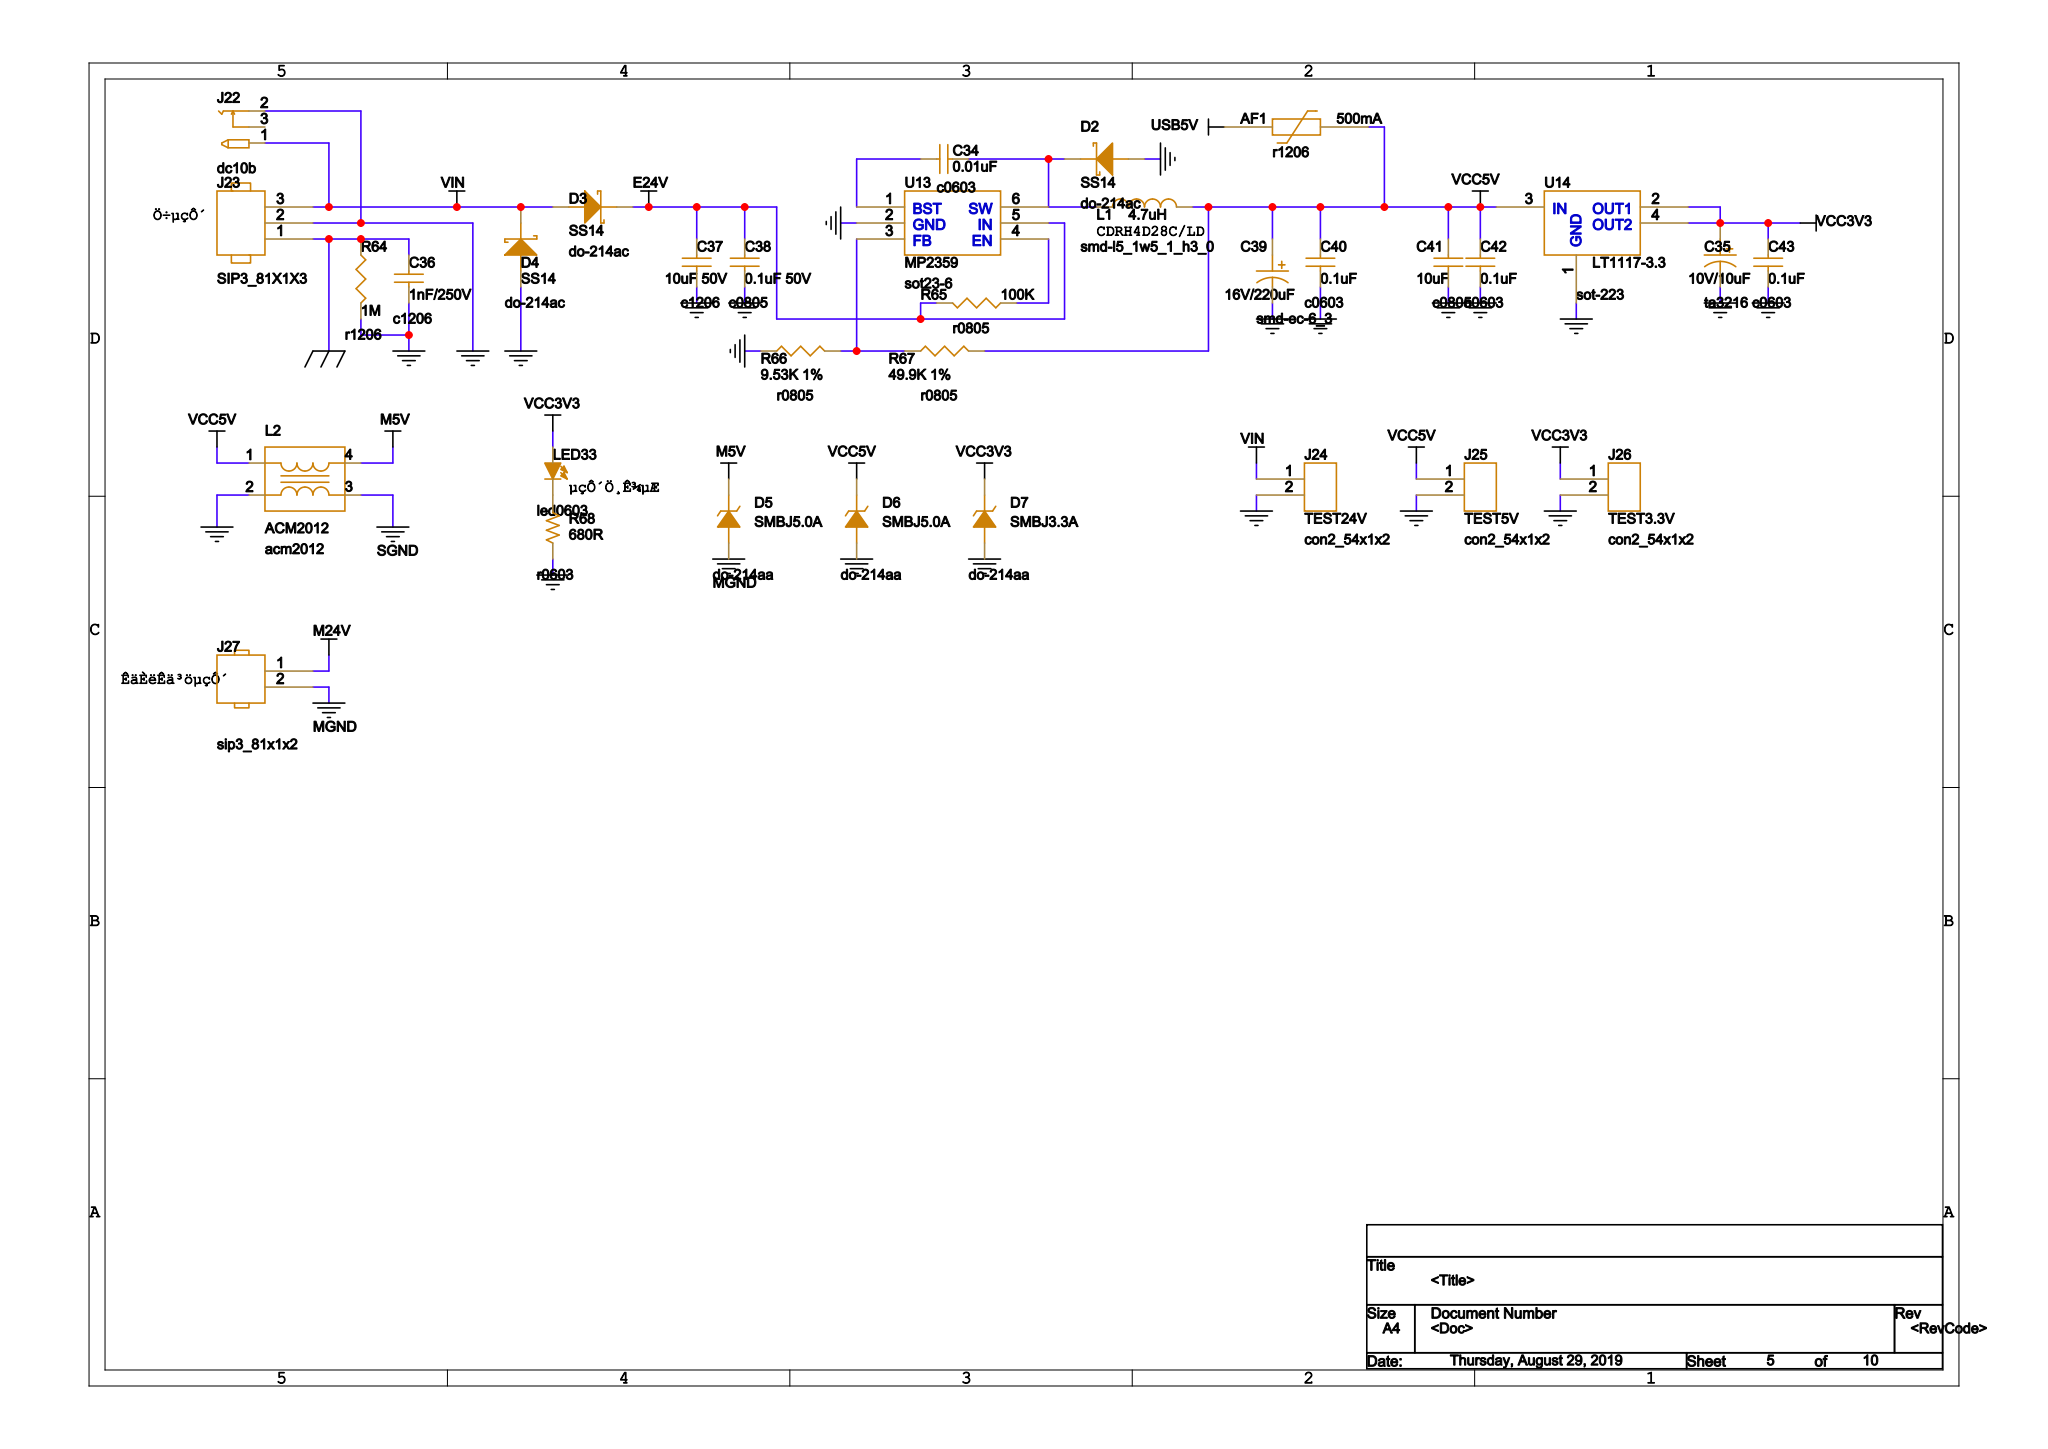Circuit board | Cadence Allegro | 380 parts | 375 nets | one sheet of the schematic
Parts on this sheet (reference | value | footprint):
AF1 | 500mA | R1206
C34 | 0.01uF | C0603
C36 | 1nF/250V | C1206
C37 | 10uF 50V | C1206
C38 | 0.1uF 50V | C0805
C39 | 16V/220uF | SMD-EC-6_3
C40 | 0.1uF | C0603
C41 | 10uF | C0805
C42 | 0.1uF | C0603
C43 | 0.1uF | C0603
D2 | SS14 | DO-214AC
D3 | SS14 | DO-214AC
D4 | SS14 | DO-214AC
D5 | SMBJ5.0A | DO-214AA
D6 | SMBJ5.0A | DO-214AA
D7 | SMBJ3.3A | DO-214AA
J22 | DC_SOCKET | DC10B
J23 | SIP3-3.81 | SIP3_81X1X3
J24 | TEST24V | CON2_54X1X2
J25 | TEST5V | CON2_54X1X2
J26 | TEST3.3V | CON2_54X1X2
J27 | HEADER 2 | SIP3_81X1X2
L1 | 4.7uH | SMD-L5_1W5_1_H3_0
L2 | ACM2012 | ACM2012
LED33 | LED | LED0603
R64 | 1M | R1206
R65 | 100K | R0805
R66 | 9.53K 1% | R0805
R67 | 49.9K 1% | R0805
R68 | 680R | R0603
U13 | MP2359 | SOT23-6
U14 | LT1117-3.3 | SOT-223
Nets of these parts (net: part-pin ...):
GND: C36-2 C37-2 C38-2 C39-2 C40-2 C41-2 C42-2 C43-2 D2-1 D4-1 D6-1 D7-1 J22-2 J23-2 J24-2 J25-2 J26-2 L2-2 R64-2 R66-1 R68-2 U13-2 U14-1
GND_EARTH: C36-1 J23-1 R64-1
M24V: J27-1
VCC3V3: C43-1 D7-2 J26-1 LED33-1 U14-2 U14-4
USB5V: AF1-1
VIN: D3-1 D4-2 J22-1 J23-3 J24-1
3: J22-3
VCC5V: AF1-2 C39-1 C40-1 C41-1 C42-1 D6-2 J25-1 L1-2 L2-1 R67-2 U14-3
N16545961: LED33-2 R68-1
SGND: L2-3
MGND: D5-1 J27-2
N440655: C34-1 U13-1
N440715: R65-1 U13-4
N440803: R66-2 R67-1 U13-3
E24V: C37-1 C38-1 D3-2 R65-2 U13-5
N440479: C34-2 D2-2 L1-1 U13-6
M5V: D5-2 L2-4